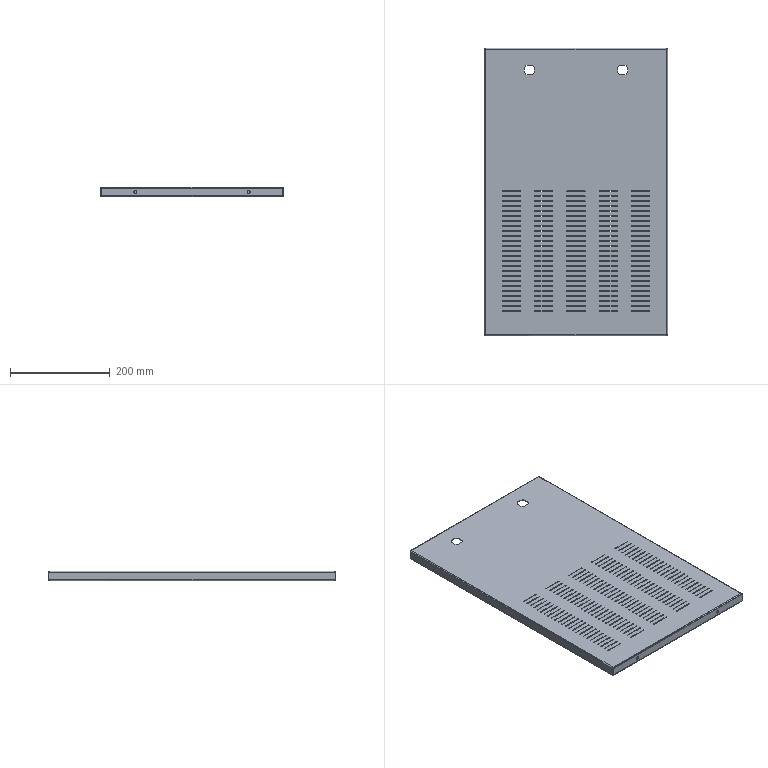Part | SolidWorks | features Cut 3, EdgeFlange 2, LPattern 2, FlatPattern 1, ICE 1, SMBaseFlange 1, SheetMetal 1 | 1 solid | 715 faces | box 367 x 577 x 20 mm | volume 391645 mm3 | cylinder 403 | plane 296 | spline 16 | commonest cylinder face diameters 1.5 x375 1.473 x8 4.473 x8 22 x8 6 x4